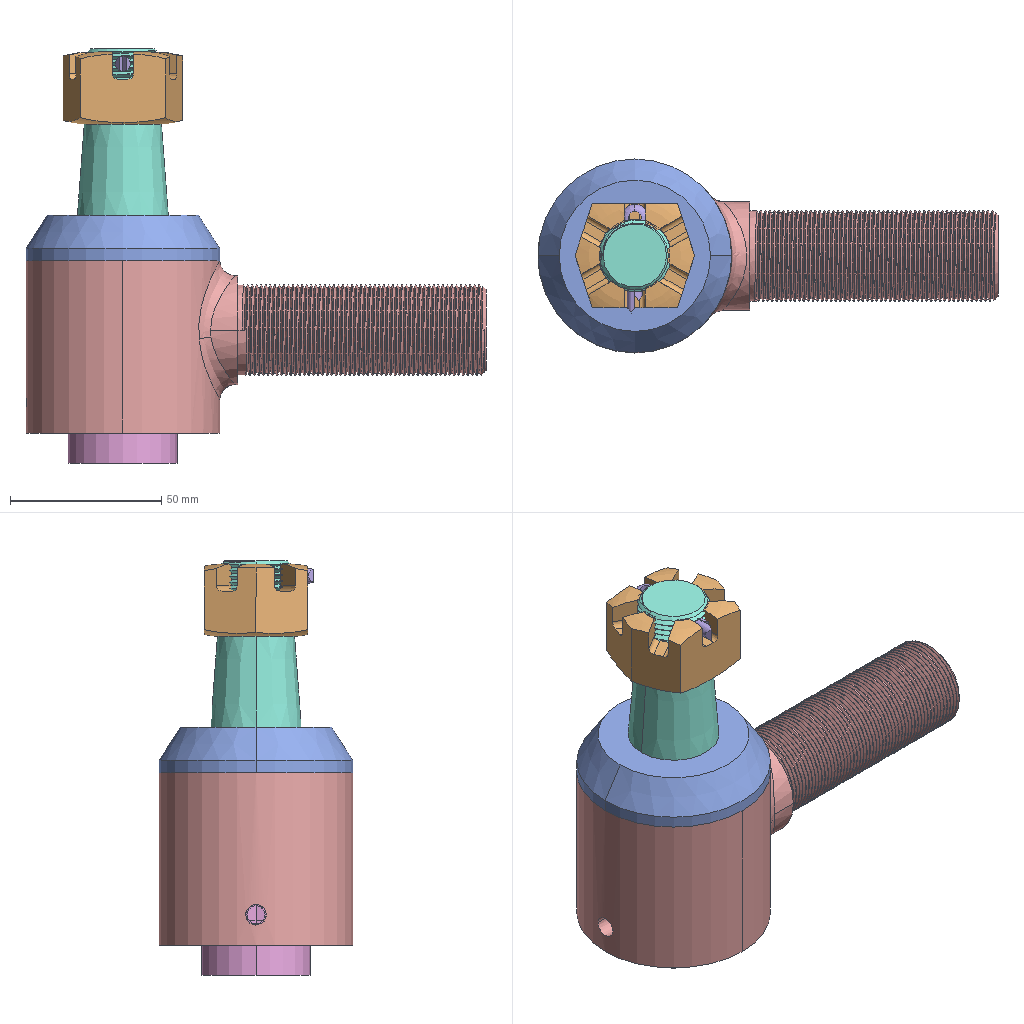Assembly | SolidWorks | 7 different items | 7 placed | box 152 x 64 x 137 mm
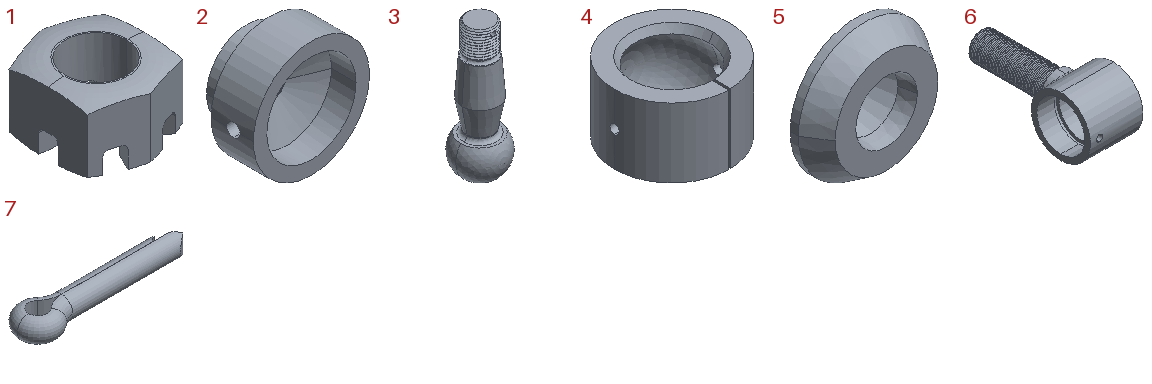Parts list (item | quantity | size | volume | features):
1 | x1 | 34.3 x 39.5 x 23.9 mm | 15247 mm3 | features CirPattern 1, Extrusion 1, Fillet 1, HoleWzd 1, ICE 1, RefAxis 1, RevCut 1
2 | x1 | 52 x 29 x 52 mm | 32471 mm3 | features HoleWzd 1, ICE 1, Revolution 1
3 | x1 | 40 x 40 x 108 mm | 69235 mm3 | features Chamfer 1, Helix 1, ICE 1, Revolution 1, SweepCut 1
4 | x1 | 50 x 49.995 x 30 mm | 27277 mm3 | features ICE 2, Revolution 1
5 | x1 | 64 x 26 x 64 mm | 21380 mm3 | features Revolution 1
6 | x1 | 57 x 152 x 64 mm | 133445 mm3 | features ICE 2, Chamfer 1, Fillet 1, Helix 1, HoleWzd 1, Revolution 1, SweepCut 1
7 | x1 | 36 x 9.2 x 5 mm | 667.949 mm3 | features Cut 1, Sweep 1
Mates (type | each side: item.copy, entity, surface, feature):
Coincident | 6.1 face plane Revolve1 | 5.1 face plane Revolve1 | 2 times
Coincident | 6.1 plane | 4.1 plane
Coincident | 6.1 face plane Revolve1 | 4.1 face plane Revolve1
Concentric | 6.1 face cylinder Revolve1 | 4.1 face cylinder Revolve1
Coincident | 4.1 face plane Revolve1 | 2.1 face plane Revolve1
Coincident | 6.1 plane | 2.1 plane
Concentric | 6.1 face cylinder Revolve1 | 2.1 face cylinder Revolve1
Coincident | 6.1 plane | 5.1 plane
Concentric | 6.1 face cylinder Revolve1 | 5.1 face cone Revolve1
Concentric | 4.1 face sphere Revolve1 | 3.1 face sphere Revolve2
PlanarAngleDim | 3.1 plane | 1.1 plane
Coincident | 3.1 face plane Revolve2 | 1.1 face plane Boss-Extrude1
Concentric | 3.1 face cylinder Cut-Extrude1 | 7.1 face cylinder Body
DistanceDim | 7.1 plane | 3.1 plane